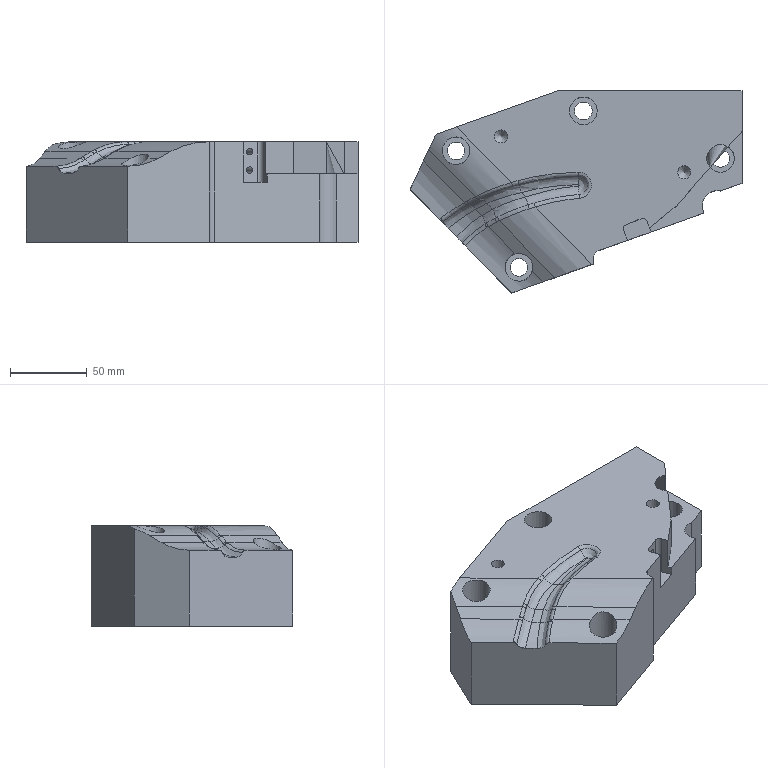Part | NX | features 23 2 | 1 solid | 99 faces | box 216.494 x 131.72 x 65.4 mm | volume 1138689 mm3 | plane 36 | cylinder 29 | spline 25 | torus 5 | cone 4 | commonest cylinder face diameters 15 x6 18 x5 11.5 x4 4.3 x2 6 x2 8.5 x2